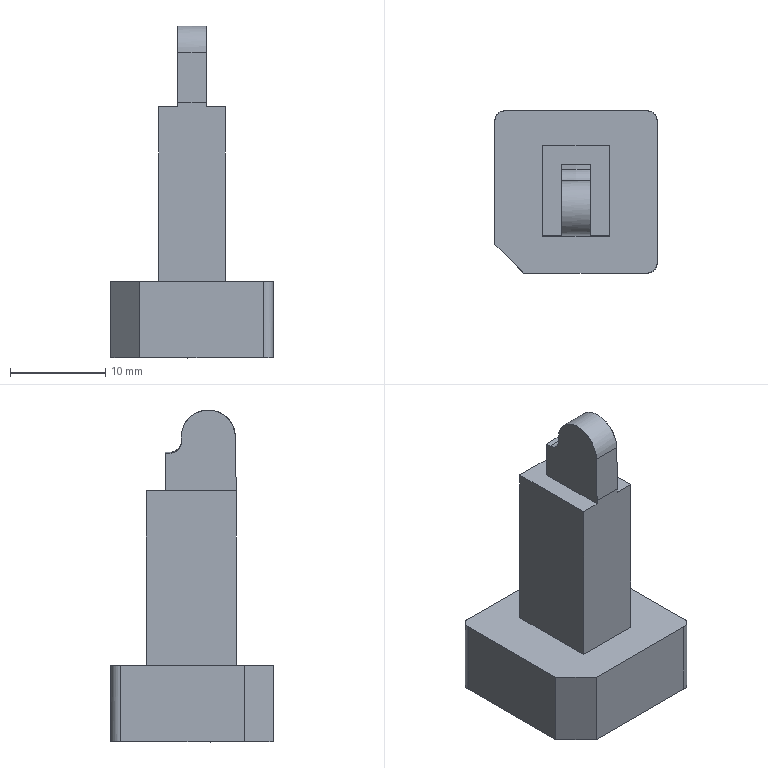NC program | PowerMill | posted with a generic post | part box 17 x 17 x 34.811 mm
Lines 14457 to 15230 of 35253:
N14554 M6
N14555 S18000 M03
N14556 G00 G90 X0.0 Y0.0
N14557 G43 Z10.798 H14
N14558
N14559 G05 P10000 R8
N14560 X2.9016 Y-3.9127
N14561 Z0.8984
N14562 G01 Z-0.3016 F1200.0
N14563 X2.8751 Y-3.8463 F2000.0
N14564 X2.8414 Y-3.7833
N14565 X2.8009 Y-3.7245
N14566 X2.7541 Y-3.6705
N14567 X2.7015 Y-3.6221
N14568 X2.6439 Y-3.5798
N14569 X2.582 Y-3.5442
N14570 X2.5165 Y-3.5158
N14571 X2.4482 Y-3.4948
N14572 X2.378 Y-3.4816
N14573 X2.3067 Y-3.4763
N14574 X2.2353 Y-3.479
N14575 X2.1646 Y-3.4896
N14576 X2.0956 Y-3.508
N14577 X2.0913 Y-3.5094
N14578 X2.0196 Y-3.5335
N14579 X1.935 Y-3.558
N14580 X1.861 Y-3.5731
N14581 X1.7759 Y-3.5869
N14582 X1.6905 Y-3.5984
N14583 X1.6048 Y-3.6064
N14584 X1.5186 Y-3.6099
N14585 X1.4322 Y-3.6102
N14586 X1.3457 Y-3.6093
N14587 X1.2593 Y-3.6087
N14588 X1.173 Y-3.6086
N14589 X-0.307 Y-3.6083
N14590 X-1.5504 Y-3.6069
N14591 X-1.6606 Y-3.6026
N14592 X-1.7723 Y-3.5904
N14593 X-1.8848 Y-3.5701
N14594 X-1.9976 Y-3.5416
N14595 X-2.1099 Y-3.5051
N14596 X-2.221 Y-3.4607
N14597 X-2.33 Y-3.4085
N14598 X-2.4359 Y-3.3489
N14599 X-2.5297 Y-3.2881
N14600 X-2.6248 Y-3.2174
N14601 X-2.7156 Y-3.1401
N14602 X-2.8014 Y-3.0565
N14603 X-2.8816 Y-2.9672
N14604 X-2.9556 Y-2.873
N14605 X-3.0196 Y-2.7794
N14606 X-3.0808 Y-2.6764
N14607 X-3.1339 Y-2.5718
N14608 X-3.1789 Y-2.4664
N14609 X-3.2136 Y-2.3667
N14610 X-3.2381 Y-2.2836
N14611 X-3.2593 Y-2.1999
N14612 X-3.2766 Y-2.1154
N14613 X-3.2893 Y-2.03
N14614 X-3.2981 Y-1.9322
N14615 X-3.3018 Y-1.8219
N14616 X-3.3019 Y-1.7278
N14617 X-3.3008 Y-1.6407
N14618 X-3.2997 Y-1.5539
N14619 X-3.2965 Y-1.4653
N14620 X-3.2853 Y-1.353
N14621 X-3.2661 Y-1.2393
N14622 X-3.2386 Y-1.1245
N14623 X-3.2029 Y-1.0088
N14624 X-3.1594 Y-0.8944
N14625 X-3.1149 Y-0.796
N14626 X-3.0684 Y-0.7098
N14627 X-3.0192 Y-0.6338
N14628 X-2.9764 Y-0.5739
N14629 X-2.9331 Y-0.5143
N14630 X-2.8889 Y-0.4555
N14631 X-2.8426 Y-0.3983
N14632 X-2.7926 Y-0.3443
N14633 X-2.7388 Y-0.2938
N14634 X-2.6837 Y-0.2448
N14635 X-2.6276 Y-0.1972
N14636 X-2.5426 Y-0.1328
N14637 X-2.4457 Y-0.0685
N14638 X-2.3401 Y-0.0078
N14639 X-2.2358 Y0.0436
N14640 X-2.1366 Y0.0848
N14641 X-2.0402 Y0.1172
N14642 X-1.9499 Y0.1419
N14643 X-1.8588 Y0.1627
N14644 X-1.7668 Y0.1788
N14645 X-1.6637 Y0.1909
N14646 X-1.5428 Y0.1983
N14647 X-1.4385 Y0.2005
N14648 X-1.3444 Y0.2008
N14649 X-1.2505 Y0.2005
N14650 X-1.1548 Y0.2002
N14651 X0.8185 Y0.1975
N14652 X1.5507 Y0.1972
N14653 X1.6544 Y0.1933
N14654 X1.7622 Y0.1813
N14655 X1.8739 Y0.1611
N14656 X1.9893 Y0.1322
N14657 X2.1076 Y0.0946
N14658 X2.208 Y0.0563
N14659 X2.3058 Y0.012
N14660 X2.4032 Y-0.0409
N14661 X2.501 Y-0.1028
N14662 X2.5993 Y-0.1742
N14663 X2.6925 Y-0.2508
N14664 X2.7784 Y-0.3305
N14665 X2.8591 Y-0.4163
N14666 X2.9341 Y-0.5078
N14667 X3.0032 Y-0.6044
N14668 X3.0657 Y-0.7058
N14669 X3.1214 Y-0.8113
N14670 X3.1699 Y-0.92
N14671 X3.2109 Y-1.0316
N14672 X3.2442 Y-1.1453
N14673 X3.2697 Y-1.2606
N14674 X3.2874 Y-1.3769
N14675 X3.2972 Y-1.4936
N14676 X3.3 Y-1.5974
N14677 X3.3022 Y-1.7022
N14678 X3.3029 Y-1.8212
N14679 X3.2989 Y-1.9403
N14680 X3.2898 Y-2.0396
N14681 X3.2765 Y-2.1274
N14682 X3.2581 Y-2.2141
N14683 X3.2353 Y-2.2998
N14684 X3.2084 Y-2.3846
N14685 X3.1781 Y-2.4684
N14686 X3.1357 Y-2.5677
N14687 X3.0838 Y-2.6695
N14688 X3.0214 Y-2.7749
N14689 X2.9546 Y-2.8732
N14690 X2.8812 Y-2.9671
N14691 X2.8016 Y-3.0559
N14692 X2.7163 Y-3.1392
N14693 X2.6255 Y-3.2166
N14694 X2.5297 Y-3.2879
N14695 X2.4294 Y-3.3525
N14696 X2.325 Y-3.4103
N14697 X2.2171 Y-3.4609
N14698 X2.106 Y-3.5043
N14699 X2.0913 Y-3.5094
N14700 X2.0478 Y-3.5263
N14701 X1.9916 Y-3.545 Z-0.3017
N14702 X1.9468 Y-3.5583
N14703 X1.9017 Y-3.5701 Z-0.3018
N14704 X1.8559 Y-3.579
N14705 X1.7465 Y-3.5975 Z-0.302
N14706 X1.6366 Y-3.6124 Z-0.3021
N14707 X1.5261 Y-3.6217 Z-0.3022
N14708 X1.4151 Y-3.6257 Z-0.3023
N14709 X1.3041 Y-3.6275 Z-0.3024
N14710 X1.1931 Y-3.629 Z-0.3025
N14711 X0.7459 Y-3.639 Z-0.303
N14712 X0.1167 Y-3.657 Z-0.3037
N14713 X-0.3503 Y-3.6667 Z-0.3041
N14714 X-1.1718 Y-3.6853 Z-0.305
N14715 X-1.5566 Y-3.6938 Z-0.3054
N14716 X-1.6463 Y-3.6921 Z-0.3055
N14717 X-1.7357 Y-3.6845 Z-0.3056
N14718 X-1.8378 Y-3.6699
N14719 X-1.9534 Y-3.6464 Z-0.3058
N14720 X-2.0677 Y-3.6159 Z-0.3059
N14721 X-2.1667 Y-3.5829 Z-0.3061
N14722 X-2.2515 Y-3.5485 Z-0.3063
N14723 X-2.3617 Y-3.4957 Z-0.3065
N14724 X-2.4608 Y-3.4404 Z-0.3068
N14725 X-2.5503 Y-3.3822 Z-0.3069
N14726 X-2.6341 Y-3.3193 Z-0.307
N14727 X-2.7184 Y-3.2495 Z-0.3072
N14728 X-2.8017 Y-3.1719 Z-0.3076
N14729 X-2.8761 Y-3.0927 Z-0.308
N14730 X-2.9429 Y-3.0115 Z-0.3083
N14731 X-3.0047 Y-2.9264 Z-0.3084
N14732 X-3.06 Y-2.8426 Z-0.3087
N14733 X-3.1015 Y-2.7717 Z-0.3092
N14734 X-3.1221 Y-2.7308 Z-0.3093
N14735 X-3.1411 Y-2.6928 Z-0.3098
N14736 X-3.1631 Y-2.6502 Z-0.3111
N14737 X-3.1977 Y-2.5825 Z-0.3135
N14738 X-3.2198 Y-2.5361 Z-0.315
N14739 X-3.236 Y-2.497 Z-0.3159
N14740 X-3.2487 Y-2.4566 Z-0.3163
N14741 X-3.2728 Y-2.3617 Z-0.3169
N14742 X-3.2881 Y-2.2719 Z-0.3173
N14743 X-3.2952 Y-2.1889 Z-0.3176
N14744 X-3.2977 Y-2.1054 Z-0.3179
N14745 X-3.3013 Y-1.8637 Z-0.3183
N14746 X-3.3017 Y-1.622 Z-0.319
N14747 Y-1.3817 Z-0.3195
N14748 X-3.298 Y-1.265 Z-0.3197
N14749 X-3.2863 Y-1.143 Z-0.3202
N14750 X-3.2669 Y-1.0212 Z-0.3205
N14751 X-3.2412 Y-0.9066 Z-0.3207
N14752 X-3.2258 Y-0.8515 Z-0.3206
N14753 X-3.2048 Y-0.7959 Z-0.3197
N14754 X-3.1714 Y-0.7258 Z-0.3177
N14755 X-3.1321 Y-0.6469 Z-0.3161
N14756 X-3.1075 Y-0.5963 Z-0.3159
N14757 X-3.0769 Y-0.5454 Z-0.3152
N14758 X-3.048 Y-0.4971 Z-0.315
N14759 X-2.9865 Y-0.3994 Z-0.3151
N14760 X-2.9167 Y-0.3033 Z-0.3152
N14761 X-2.8391 Y-0.21 Z-0.3154
N14762 X-2.7545 Y-0.1208 Z-0.3157
N14763 X-2.6724 Y-0.0441 Z-0.316
N14764 X-2.5801 Y0.0336 Z-0.3164
N14765 X-2.4999 Y0.0935 Z-0.3168
N14766 X-2.4164 Y0.1485 Z-0.3172
N14767 X-2.3114 Y0.2099 Z-0.3177
N14768 X-2.2085 Y0.2615 Z-0.3181
N14769 X-2.1078 Y0.3038 Z-0.3184
N14770 X-2.0091 Y0.3371 Z-0.3186
N14771 X-1.9189 Y0.3617 Z-0.3188
N14772 X-1.828 Y0.3829 Z-0.319
N14773 X-1.7362 Y0.3998 Z-0.3193
N14774 X-1.6384 Y0.4123 Z-0.3196
N14775 X-1.5372 Y0.4198 Z-0.3199
N14776 X-1.4435 Y0.4233 Z-0.3202
N14777 X-1.3497 Y0.425 Z-0.3204
N14778 X-1.256 Y0.4259 Z-0.3206
N14779 X-1.1625 Y0.427 Z-0.3209
N14780 X-0.7326 Y0.4357 Z-0.3219
N14781 X-0.1421 Y0.4514 Z-0.3235
N14782 X0.3613 Y0.462 Z-0.3248
N14783 X1.3883 Y0.4864 Z-0.3278
N14784 X1.4783 Y0.4881 Z-0.3281
N14785 X1.5685 Y0.488 Z-0.3284
N14786 X1.6585 Y0.485 Z-0.3287
N14787 X1.7483 Y0.4776 Z-0.329
N14788 X1.8373 Y0.4647 Z-0.3293
N14789 X1.9256 Y0.4469 Z-0.3297
N14790 X2.013 Y0.4256 Z-0.33
N14791 X2.1207 Y0.3936 Z-0.3305
N14792 X2.227 Y0.3538 Z-0.3309
N14793 X2.332 Y0.306 Z-0.3313
N14794 X2.4352 Y0.2502 Z-0.3317
N14795 X2.5354 Y0.1873 Z-0.3321
N14796 X2.6313 Y0.1175 Z-0.3324
N14797 X2.7231 Y0.041 Z-0.3329
N14798 X2.8103 Y-0.042 Z-0.3334
N14799 X2.8922 Y-0.1312 Z-0.334
N14800 X2.9686 Y-0.2259 Z-0.3348
N14801 X3.0403 Y-0.3249 Z-0.3365
N14802 X3.0898 Y-0.4002 Z-0.3384
N14803 X3.1269 Y-0.4675 Z-0.3394
N14804 X3.1692 Y-0.5608 Z-0.3399
N14805 X3.2092 Y-0.6673 Z-0.3401
N14806 X3.2432 Y-0.7797 Z-0.3404
N14807 X3.2696 Y-0.8943 Z-0.3407
N14808 X3.2882 Y-1.0108 Z-0.341
N14809 X3.2989 Y-1.1286 Z-0.3413
N14810 X3.3017 Y-1.2473 Z-0.3416
N14811 Y-2.1997 Z-0.3439
N14812 X3.2978 Y-2.3244 Z-0.3443
N14813 X3.2859 Y-2.4476 Z-0.3447
N14814 X3.2663 Y-2.5688 Z-0.3451
N14815 X3.2391 Y-2.6875 Z-0.3454
N14816 X3.2045 Y-2.803 Z-0.3457
N14817 X3.1628 Y-2.9151 Z-0.346
N14818 X3.114 Y-3.0232 Z-0.3462
N14819 X3.0586 Y-3.1271 Z-0.3463
N14820 X2.9965 Y-3.2267
N14821 X2.926 Y-3.3248 Z-0.3464
N14822 X2.8479 Y-3.4199 Z-0.3466
N14823 X2.7631 Y-3.5105 Z-0.347
N14824 X2.6734 Y-3.5949 Z-0.3474
N14825 X2.5798 Y-3.6721 Z-0.3479
N14826 X2.4837 Y-3.7414 Z-0.3484
N14827 X2.3859 Y-3.8025 Z-0.3489
N14828 X2.2875 Y-3.855 Z-0.3493
N14829 X2.2596 Y-3.8682 Z-0.3494
N14830 X2.1901 Y-3.9012 Z-0.3496
N14831 X2.1164 Y-3.9305 Z-0.3497
N14832 X2.0149 Y-3.9647 Z-0.35
N14833 X1.9407 Y-3.9858 Z-0.3501
N14834 X1.8657 Y-4.0034 Z-0.3503
N14835 X1.7538 Y-4.0228 Z-0.3506
N14836 X1.6322 Y-4.0363 Z-0.3508
N14837 X1.494 Y-4.0442 Z-0.3511
N14838 X1.3253 Y-4.0467 Z-0.3515
N14839 X1.0775 Y-4.046 Z-0.3521
N14840 X0.6713 Y-4.0498 Z-0.353
N14841 X0.088 Y-4.0593 Z-0.3543
N14842 X-0.3656 Y-4.0635 Z-0.3553
N14843 X-1.3875 Y-4.0755 Z-0.3575
N14844 X-1.4777 Y-4.076 Z-0.3577
N14845 X-1.5679 Y-4.0747 Z-0.3579
N14846 X-1.658 Y-4.0705 Z-0.3581
N14847 X-1.7478 Y-4.0623 Z-0.3582
N14848 X-1.843 Y-4.048 Z-0.3584
N14849 X-1.9311 Y-4.0292 Z-0.3586
N14850 X-2.0183 Y-4.006 Z-0.3588
N14851 X-2.1044 Y-3.9794 Z-0.359
N14852 X-2.2124 Y-3.9389 Z-0.3592
N14853 X-2.318 Y-3.8908 Z-0.3594
N14854 X-2.4209 Y-3.8352 Z-0.3597
N14855 X-2.5183 Y-3.7739 Z-0.3599
N14856 X-2.6164 Y-3.7034 Z-0.3604
N14857 X-2.7117 Y-3.6256 Z-0.3609
N14858 X-2.7982 Y-3.5452 Z-0.3614
N14859 X-2.8742 Y-3.4647 Z-0.3619
N14860 X-2.9394 Y-3.3853 Z-0.3623
N14861 X-2.9993 Y-3.3016 Z-0.3627
N14862 X-3.0635 Y-3.1993 Z-0.363
N14863 X-3.1204 Y-3.0938 Z-0.3634
N14864 X-3.1696 Y-2.9858 Z-0.3637
N14865 X-3.211 Y-2.8759 Z-0.3639
N14866 X-3.2445 Y-2.7646 Z-0.3642
N14867 X-3.2701 Y-2.6523 Z-0.3644
N14868 X-3.2877 Y-2.5396 Z-0.3647
N14869 X-3.2974 Y-2.4268 Z-0.365
N14870 X-3.3 Y-2.3136 Z-0.3652
N14871 X-3.3036 Y-1.727 Z-0.3667
N14872 X-3.3015 Y-1.0608 Z-0.3683
N14873 X-3.2968 Y-0.948 Z-0.3685
N14874 X-3.2841 Y-0.8338 Z-0.3688
N14875 X-3.2634 Y-0.7183 Z-0.3691
N14876 X-3.2345 Y-0.6018 Z-0.3694
N14877 X-3.1972 Y-0.4849 Z-0.3697
N14878 X-3.1536 Y-0.3726 Z-0.3699
N14879 X-3.1033 Y-0.264 Z-0.3703
N14880 X-3.0464 Y-0.16 Z-0.3707
N14881 X-2.9832 Y-0.061 Z-0.3709
N14882 X-2.9141 Y0.033
N14883 X-2.8379 Y0.1234 Z-0.371
N14884 X-2.7559 Y0.2085
N14885 X-2.668 Y0.2882 Z-0.3711
N14886 X-2.574 Y0.3627 Z-0.3712
N14887 X-2.4738 Y0.4319 Z-0.3713
N14888 X-2.3735 Y0.4925 Z-0.3715
N14889 X-2.2668 Y0.5485 Z-0.3718
N14890 X-2.1585 Y0.5964 Z-0.3721
N14891 X-2.0487 Y0.6365 Z-0.3724
N14892 X-1.9369 Y0.6688 Z-0.3727
N14893 X-1.8301 Y0.6922 Z-0.373
N14894 X-1.7157 Y0.7093 Z-0.3733
N14895 X-1.5869 Y0.721 Z-0.3735
N14896 X-1.435 Y0.7275 Z-0.3738
N14897 X-1.2322 Y0.7298 Z-0.3743
N14898 X-0.8657 Y0.7323 Z-0.3752
N14899 X0.3671 Y0.7445 Z-0.3781
N14900 X1.5479 Y0.7569 Z-0.3809
N14901 X1.6453 Y0.7541 Z-0.3812
N14902 X1.7473 Y0.7441 Z-0.3815
N14903 X1.86 Y0.7259 Z-0.3817
N14904 X1.9799 Y0.6987 Z-0.382
N14905 X2.0924 Y0.6658 Z-0.3823
N14906 X2.1914 Y0.6303 Z-0.3825
N14907 X2.2744 Y0.5948 Z-0.3827
N14908 X2.3553 Y0.5544 Z-0.383
N14909 X2.4444 Y0.504 Z-0.3834
N14910 X2.546 Y0.4389 Z-0.384
N14911 X2.6404 Y0.3705 Z-0.3847
N14912 X2.7173 Y0.3076 Z-0.3852
N14913 X2.7834 Y0.2462 Z-0.3856
N14914 X2.8452 Y0.1803 Z-0.3859
N14915 X2.9239 Y0.0858 Z-0.3862
N14916 X2.9958 Y-0.0128 Z-0.3865
N14917 X3.0605 Y-0.1149 Z-0.3868
N14918 X3.1176 Y-0.2198 Z-0.3871
N14919 X3.167 Y-0.3269 Z-0.3874
N14920 X3.2086 Y-0.4357 Z-0.3876
N14921 X3.2422 Y-0.5456 Z-0.3879
N14922 X3.2677 Y-0.6562 Z-0.3882
N14923 X3.2853 Y-0.7671 Z-0.3884
N14924 X3.295 Y-0.8781 Z-0.3887
N14925 X3.2987 Y-0.9897 Z-0.389
N14926 X3.3018 Y-1.1756 Z-0.3895
N14927 X3.3033 Y-1.3615 Z-0.3899
N14928 X3.3039 Y-1.5475 Z-0.3904
N14929 X3.3037 Y-1.7631 Z-0.3909
N14930 X3.303 Y-1.9491 Z-0.3913
N14931 X3.3018 Y-2.135 Z-0.3917
N14932 X3.3 Y-2.321 Z-0.3922
N14933 X3.2974 Y-2.507 Z-0.3926
N14934 X3.2935 Y-2.607 Z-0.3929
N14935 X3.282 Y-2.7094 Z-0.3931
N14936 X3.2622 Y-2.8155 Z-0.3934
N14937 X3.2337 Y-2.9257 Z-0.3937
N14938 X3.196 Y-3.0405 Z-0.394
N14939 X3.1486 Y-3.1604 Z-0.3943
N14940 X3.1005 Y-3.2638 Z-0.3945
N14941 X3.0448 Y-3.3647 Z-0.3948
N14942 X2.9814 Y-3.4633 Z-0.3951
N14943 X2.9103 Y-3.5592 Z-0.3954
N14944 X2.8317 Y-3.6519 Z-0.3957
N14945 X2.7457 Y-3.7411 Z-0.396
N14946 X2.687 Y-3.7959 Z-0.3962
N14947 X2.6257 Y-3.8478 Z-0.3963
N14948 X2.5588 Y-3.8991 Z-0.3965
N14949 X2.4701 Y-3.9606 Z-0.3968
N14950 X2.4019 Y-4.0027 Z-0.397
N14951 X2.3404 Y-4.0357 Z-0.3972
N14952 X2.2407 Y-4.0857 Z-0.3974
N14953 X2.1331 Y-4.1311 Z-0.3977
N14954 X2.0196 Y-4.1705 Z-0.3979
N14955 X1.9044 Y-4.2021 Z-0.3982
N14956 X1.7905 Y-4.2254 Z-0.3984
N14957 X1.68 Y-4.2403 Z-0.3987
N14958 X1.5741 Y-4.2472 Z-0.3989
N14959 X1.4685 Y-4.2487 Z-0.3991
N14960 X0.3105 Y-4.2597 Z-0.4016
N14961 X-1.0396 Y-4.2704 Z-0.4045
N14962 X-1.3875 Y-4.2737 Z-0.4052
N14963 X-1.4804 Y-4.2742 Z-0.4054
N14964 X-1.5734 Y-4.2729 Z-0.4057
N14965 X-1.6726 Y-4.2679 Z-0.406
N14966 X-1.7789 Y-4.2567 Z-0.4063
N14967 X-1.8702 Y-4.2411 Z-0.4065
N14968 X-1.9604 Y-4.2202 Z-0.4067
N14969 X-2.0495 Y-4.1947 Z-0.4068
N14970 X-2.1374 Y-4.1651 Z-0.4069
N14971 X-2.2475 Y-4.1209 Z-0.4072
N14972 X-2.3547 Y-4.0694 Z-0.4076
N14973 X-2.459 Y-4.0104 Z-0.408
N14974 X-2.5552 Y-3.9476 Z-0.4085
N14975 X-2.6469 Y-3.879 Z-0.409
N14976 X-2.7329 Y-3.8048 Z-0.4094
N14977 X-2.8178 Y-3.7211 Z-0.4096
N14978 X-2.8962 Y-3.6327 Z-0.4099
N14979 X-2.9676 Y-3.5403 Z-0.4102
N14980 X-3.032 Y-3.4442 Z-0.4104
N14981 X-3.0822 Y-3.3575 Z-0.4107
N14982 X-3.1382 Y-3.2481 Z-0.411
N14983 X-3.1799 Y-3.1535 Z-0.4112
N14984 X-3.2116 Y-3.0651 Z-0.4114
N14985 X-3.2378 Y-2.9778 Z-0.4116
N14986 X-3.2598 Y-2.8885 Z-0.4118
N14987 X-3.2775 Y-2.7948 Z-0.4121
N14988 X-3.2907 Y-2.6926 Z-0.4123
N14989 X-3.299 Y-2.5745 Z-0.4126
N14990 X-3.3021 Y-2.4384 Z-0.413
N14991 X-3.302 Y-2.3197 Z-0.4132
N14992 X-3.3016 Y-2.2106 Z-0.4134
N14993 Y-2.0981 Z-0.4136
N14994 X-3.3017 Y-0.8977 Z-0.4165
N14995 X-3.2977 Y-0.7794 Z-0.4167
N14996 X-3.2858 Y-0.6615 Z-0.417
N14997 X-3.2659 Y-0.5441 Z-0.4173
N14998 X-3.2382 Y-0.4277 Z-0.4176
N14999 X-3.2026 Y-0.3129 Z-0.4179
N15000 X-3.1593 Y-0.2001 Z-0.4182
N15001 X-3.1084 Y-0.0901 Z-0.4185
N15002 X-3.0503 Y0.0168 Z-0.4187
N15003 X-2.9852 Y0.1197 Z-0.419
N15004 X-2.9143 Y0.2169 Z-0.4192
N15005 X-2.8372 Y0.3092 Z-0.4195
N15006 X-2.7544 Y0.3958 Z-0.4199
N15007 X-2.6663 Y0.4765 Z-0.4202
N15008 X-2.5735 Y0.5507 Z-0.4204
N15009 X-2.4765 Y0.6182 Z-0.4206
N15010 X-2.3751 Y0.6791 Z-0.4207
N15011 X-2.2678 Y0.7343 Z-0.4208
N15012 X-2.1565 Y0.7826 Z-0.421
N15013 X-2.0425 Y0.8234 Z-0.4212
N15014 X-1.9274 Y0.8562 Z-0.4214
N15015 X-1.8123 Y0.8809 Z-0.4216
N15016 X-1.6982 Y0.8975 Z-0.4219
N15017 X-1.586 Y0.9059 Z-0.4221
N15018 X-1.4744 Y0.9083 Z-0.4224
N15019 X-0.9294 Y0.9139 Z-0.4237
N15020 X-0.317 Y0.918 Z-0.4251
N15021 X0.7133 Y0.9251 Z-0.4276
N15022 X1.4557 Y0.9316 Z-0.4294
N15023 X1.5869 Y0.9296 Z-0.4297
N15024 X1.7121 Y0.9203 Z-0.43
N15025 X1.832 Y0.904 Z-0.4303
N15026 X1.9472 Y0.8805 Z-0.4306
N15027 X2.0581 Y0.85 Z-0.431
N15028 X2.1655 Y0.8125 Z-0.4314
N15029 X2.2707 Y0.7679 Z-0.4318
N15030 X2.3778 Y0.714 Z-0.4322
N15031 X2.4806 Y0.6534 Z-0.4325
N15032 X2.5787 Y0.5863 Z-0.4328
N15033 X2.6717 Y0.5131 Z-0.433
N15034 X2.7592 Y0.434 Z-0.4332
N15035 X2.8412 Y0.3493 Z-0.4335
N15036 X2.9172 Y0.2595 Z-0.4338
N15037 X2.9888 Y0.1625 Z-0.4341
N15038 X3.0536 Y0.0613 Z-0.4344
N15039 X3.1113 Y-0.0434 Z-0.4347
N15040 X3.1616 Y-0.151 Z-0.4349
N15041 X3.2041 Y-0.261 Z-0.4352
N15042 X3.2389 Y-0.3726 Z-0.4355
N15043 X3.2658 Y-0.4855 Z-0.4357
N15044 X3.2847 Y-0.599 Z-0.436
N15045 X3.2957 Y-0.7126 Z-0.4363
N15046 X3.3005 Y-0.8269 Z-0.4365
N15047 X3.3041 Y-1.048 Z-0.4371
N15048 X3.3028 Y-1.3477 Z-0.4377
N15049 X3.3017 Y-1.664 Z-0.4385
N15050 Y-2.2037 Z-0.4397
N15051 X3.2993 Y-2.6465 Z-0.4408
N15052 X3.2985 Y-2.7111 Z-0.4409
N15053 X3.2938 Y-2.7754 Z-0.4411
N15054 X3.2855 Y-2.8405 Z-0.4412
N15055 X3.2709 Y-2.9255 Z-0.4414
N15056 X3.2482 Y-3.0298 Z-0.4417
N15057 X3.2287 Y-3.1042 Z-0.4418
N15058 X3.2095 Y-3.1658 Z-0.442
N15059 X3.1874 Y-3.2265 Z-0.4421
N15060 X3.1382 Y-3.3444 Z-0.4424
N15061 X3.0841 Y-3.4546 Z-0.4427
N15062 X3.0245 Y-3.5587 Z-0.443
N15063 X2.9608 Y-3.6544 Z-0.4433
N15064 X2.8894 Y-3.7475 Z-0.4436
N15065 X2.8106 Y-3.837 Z-0.4438
N15066 X2.7253 Y-3.9221 Z-0.4441
N15067 X2.6347 Y-4.001 Z-0.4444
N15068 X2.5402 Y-4.0731 Z-0.4447
N15069 X2.4427 Y-4.1375 Z-0.4449
N15070 X2.4152 Y-4.1541 Z-0.445
N15071 X2.3065 Y-4.214 Z-0.4453
N15072 X2.2006 Y-4.264 Z-0.4455
N15073 X2.0968 Y-4.3047 Z-0.4458
N15074 X2.0049 Y-4.3342 Z-0.446
N15075 X1.9118 Y-4.359 Z-0.4462
N15076 X1.8177 Y-4.3791 Z-0.4464
N15077 X1.7226 Y-4.3938 Z-0.4466
N15078 X1.6149 Y-4.4041 Z-0.4469
N15079 X1.4917 Y-4.4092 Z-0.4471
N15080 X1.3845 Y-4.41 Z-0.4474
N15081 X1.2854 Y-4.4095 Z-0.4476
N15082 X1.1889 Y-4.4094 Z-0.4478
N15083 X0.9803 Y-4.4105 Z-0.4483
N15084 X0.7717 Y-4.4124 Z-0.4488
N15085 X0.5631 Y-4.4144 Z-0.4492
N15086 X0.3247 Y-4.4168 Z-0.4498
N15087 X0.1161 Y-4.4187 Z-0.4502
N15088 X-0.0925 Y-4.4203 Z-0.4507
N15089 X-0.3011 Y-4.4213 Z-0.4511
N15090 X-1.4563 Y-4.4278 Z-0.4537
N15091 X-1.5595 Y-4.4282 Z-0.4539
N15092 X-1.6625 Y-4.4244 Z-0.4542
N15093 X-1.7697 Y-4.4125 Z-0.4544
N15094 X-1.882 Y-4.3924 Z-0.4547
N15095 X-2.0003 Y-4.3633 Z-0.455
N15096 X-2.1112 Y-4.3291 Z-0.4553
N15097 X-2.2197 Y-4.2875 Z-0.4556
N15098 X-2.3258 Y-4.2383 Z-0.4559
N15099 X-2.429 Y-4.1818 Z-0.4562
N15100 X-2.5288 Y-4.1179 Z-0.4565
N15101 X-2.6249 Y-4.0471 Z-0.4567
N15102 X-2.7167 Y-3.9694 Z-0.457
N15103 X-2.8038 Y-3.8853 Z-0.4573
N15104 X-2.8821 Y-3.7991 Z-0.4575
N15105 X-2.9549 Y-3.7072 Z-0.4578
N15106 X-3.0217 Y-3.6099 Z-0.458
N15107 X-3.0821 Y-3.508 Z-0.4583
N15108 X-3.1354 Y-3.4022 Z-0.4586
N15109 X-3.1747 Y-3.3108 Z-0.4588
N15110 X-3.2085 Y-3.2196 Z-0.459
N15111 X-3.2375 Y-3.1252 Z-0.4592
N15112 X-3.2615 Y-3.0257 Z-0.4595
N15113 X-3.2804 Y-2.9179 Z-0.4597
N15114 X-3.2937 Y-2.7983 Z-0.46
N15115 X-3.3011 Y-2.6676 Z-0.4603
N15116 X-3.3036 Y-2.5423 Z-0.4606
N15117 X-3.3038 Y-2.4223 Z-0.4609
N15118 X-3.3033 Y-2.3054 Z-0.4611
N15119 X-3.303 Y-2.1853 Z-0.4614
N15120 X-3.3016 Y-0.7345 Z-0.4647
N15121 X-3.2976 Y-0.6215 Z-0.4649
N15122 X-3.2857 Y-0.5077 Z-0.4652
N15123 X-3.2657 Y-0.3932 Z-0.4654
N15124 X-3.2376 Y-0.2784 Z-0.4657
N15125 X-3.2014 Y-0.1637 Z-0.466
N15126 X-3.1571 Y-0.0497 Z-0.4663
N15127 X-3.1048 Y0.0629 Z-0.4665
N15128 X-3.0479 Y0.1672 Z-0.4668
N15129 X-2.9839 Y0.2677 Z-0.4671
N15130 X-2.9132 Y0.3642 Z-0.4673
N15131 X-2.8359 Y0.456 Z-0.4676
N15132 X-2.7524 Y0.5427 Z-0.4679
N15133 X-2.6632 Y0.6239 Z-0.4682
N15134 X-2.5689 Y0.699 Z-0.4684
N15135 X-2.4708 Y0.767 Z-0.4687
N15136 X-2.3694 Y0.8277 Z-0.469
N15137 X-2.2652 Y0.881 Z-0.4692
N15138 X-2.1761 Y0.9197 Z-0.4695
N15139 X-2.088 Y0.953 Z-0.4697
N15140 X-1.9984 Y0.9821 Z-0.4699
N15141 X-1.9051 Y1.007 Z-0.4701
N15142 X-1.8052 Y1.0274 Z-0.4703
N15143 X-1.6942 Y1.0429 Z-0.4706
N15144 X-1.5686 Y1.0528 Z-0.4709
N15145 X-1.4502 Y1.057 Z-0.4711
N15146 X-1.3386 Y1.0581 Z-0.4714
N15147 X-1.2307 Y1.0582 Z-0.4716
N15148 X-1.1192 Z-0.4719
N15149 X-0.3132 Y1.0615 Z-0.4737
N15150 X0.4996 Y1.0667 Z-0.4755
N15151 X0.9845 Y1.0712 Z-0.4766
N15152 X1.384 Y1.0733 Z-0.4775
N15153 X1.5593 Y1.072 Z-0.4779
N15154 X1.6704 Y1.0667 Z-0.4782
N15155 X1.7831 Y1.0534 Z-0.4784
N15156 X1.8974 Y1.0319 Z-0.4787
N15157 X2.0128 Y1.0022 Z-0.479
N15158 X2.1289 Y0.9642 Z-0.4792
N15159 X2.2377 Y0.9209 Z-0.4795
N15160 X2.3435 Y0.8705 Z-0.4798
N15161 X2.4463 Y0.8127 Z-0.48
N15162 X2.5456 Y0.7477 Z-0.4803
N15163 X2.6409 Y0.6758 Z-0.4806
N15164 X2.7317 Y0.5973 Z-0.4809
N15165 X2.8167 Y0.5135 Z-0.4811
N15166 X2.8946 Y0.4257 Z-0.4814
N15167 X2.9652 Y0.3344 Z-0.4816
N15168 X3.0283 Y0.2401 Z-0.4819
N15169 X3.085 Y0.1418 Z-0.4822
N15170 X3.1383 Y0.0343 Z-0.4824
N15171 X3.1895 Y-0.0854 Z-0.4827
N15172 X3.2095 Y-0.1414 Z-0.4829
N15173 X3.2269 Y-0.1982 Z-0.483
N15174 X3.2457 Y-0.267 Z-0.4832
N15175 X3.2687 Y-0.3653 Z-0.4834
N15176 X3.2838 Y-0.4461 Z-0.4836
N15177 X3.2923 Y-0.5075 Z-0.4837
N15178 X3.2965 Y-0.5666 Z-0.4838
N15179 X3.2973 Y-0.626 Z-0.484
N15180 X3.3015 Y-0.9821 Z-0.4848
N15181 X3.3017 Y-1.2945 Z-0.4855
N15182 Y-1.714 Z-0.4864
N15183 X3.3025 Y-2.3333 Z-0.4878
N15184 X3.2998 Y-2.7236 Z-0.4887
N15185 X3.2974 Y-2.8584 Z-0.489
N15186 X3.2934 Y-2.9164 Z-0.4892
N15187 X3.2859 Y-2.9741 Z-0.4893
N15188 X3.2741 Y-3.0443 Z-0.4895
N15189 X3.2539 Y-3.1413 Z-0.4897
N15190 X3.2324 Y-3.227 Z-0.4899
N15191 X3.214 Y-3.29 Z-0.49
N15192 X3.1951 Y-3.3451 Z-0.4902
N15193 X3.1736 Y-3.3993 Z-0.4903
N15194 X3.1218 Y-3.5153 Z-0.4906
N15195 X3.0641 Y-3.6253 Z-0.4909
N15196 X3.0105 Y-3.7142 Z-0.4911
N15197 X2.9591 Y-3.7893 Z-0.4913
N15198 X2.8954 Y-3.8717 Z-0.4915
N15199 X2.8183 Y-3.9602 Z-0.4918
N15200 X2.7327 Y-4.0471 Z-0.4921
N15201 X2.6501 Y-4.1211 Z-0.4923
N15202 X2.5729 Y-4.182 Z-0.4925
N15203 X2.4991 Y-4.2326 Z-0.4927
N15204 X2.4733 Y-4.2483 Z-0.4928
N15205 X2.371 Y-4.311 Z-0.4931
N15206 X2.2656 Y-4.3663 Z-0.4933
N15207 X2.1571 Y-4.4143 Z-0.4936
N15208 X2.0458 Y-4.4548 Z-0.4939
N15209 X1.9447 Y-4.4838 Z-0.4941
N15210 X1.8359 Y-4.507 Z-0.4943
N15211 X1.7169 Y-4.5245 Z-0.4946
N15212 X1.5842 Y-4.5364 Z-0.4949
N15213 X1.4309 Y-4.5427 Z-0.4952
N15214 X1.239 Y-4.5439 Z-0.4957
N15215 X0.9371 Y-4.5431 Z-0.4963
N15216 X0.2883 Y-4.5463 Z-0.4978
N15217 X-0.8152 Y-4.5537 Z-0.5002
N15218 X-1.5522 Y-4.5557 Z-0.5018
N15219 X-1.6608 Y-4.5517 Z-0.5021
N15220 X-1.7713 Y-4.5398 Z-0.5023
N15221 X-1.8838 Y-4.5198 Z-0.5026
N15222 X-1.998 Y-4.4914 Z-0.5028
N15223 X-2.1133 Y-4.4547 Z-0.5031
N15224 X-2.222 Y-4.4125 Z-0.5034
N15225 X-2.3278 Y-4.3635 Z-0.5036
N15226 X-2.4307 Y-4.307 Z-0.5039
N15227 X-2.5303 Y-4.2432 Z-0.5041
N15228 X-2.6262 Y-4.1724 Z-0.5044
N15229 X-2.717 Y-4.0955 Z-0.5047
N15230 X-2.8026 Y-4.0127 Z-0.5049
N15231 X-2.8825 Y-3.9242 Z-0.5052
N15232 X-2.9564 Y-3.8306 Z-0.5055
N15233 X-3.0237 Y-3.7323 Z-0.5057
N15234 X-3.0842 Y-3.6299 Z-0.506
N15235 X-3.139 Y-3.5216 Z-0.5062
N15236 X-3.1857 Y-3.4122 Z-0.5065
N15237 X-3.2242 Y-3.3022 Z-0.5068
N15238 X-3.2545 Y-3.1922 Z-0.507
N15239 X-3.2766 Y-3.0825 Z-0.5073
N15240 X-3.2907 Y-2.9735 Z-0.5075
N15241 X-3.2968 Y-2.8654 Z-0.5077
N15242 X-3.298 Y-2.757 Z-0.508
N15243 X-3.3013 Y-2.1048 Z-0.5094
N15244 X-3.3015 Y-1.7139 Z-0.5103
N15245 X-3.3036 Y-1.1977 Z-0.5114
N15246 X-3.3035 Y-0.7848 Z-0.5123
N15247 X-3.3006 Y-0.5704 Z-0.5128
N15248 X-3.2945 Y-0.4619 Z-0.5131
N15249 X-3.2805 Y-0.3511 Z-0.5133
N15250 X-3.2582 Y-0.238 Z-0.5136
N15251 X-3.2274 Y-0.1225 Z-0.5138
N15252 X-3.188 Y-0.005 Z-0.5141
N15253 X-3.1444 Y0.1033 Z-0.5144
N15254 X-3.0938 Y0.2086 Z-0.5146
N15255 X-3.0356 Y0.3112 Z-0.5149
N15256 X-2.9701 Y0.4108 Z-0.5151
N15257 X-2.8974 Y0.5067 Z-0.5154
N15258 X-2.8196 Y0.5966 Z-0.5157
N15259 X-2.7359 Y0.6813 Z-0.5159
N15260 X-2.6467 Y0.7603 Z-0.5162
N15261 X-2.5521 Y0.8334 Z-0.5165
N15262 X-2.4525 Y0.9004 Z-0.5167
N15263 X-2.3483 Y0.9608 Z-0.517
N15264 X-2.2399 Y1.0144 Z-0.5173
N15265 X-2.1278 Y1.0609 Z-0.5175
N15266 X-2.0273 Y1.0955 Z-0.5178
N15267 X-1.9114 Y1.1279 Z-0.518
N15268 X-1.7985 Y1.1517 Z-0.5183
N15269 X-1.6895 Y1.167 Z-0.5185
N15270 X-1.5848 Y1.1742 Z-0.5188
N15271 X-1.4815 Y1.1752 Z-0.519
N15272 X-0.2563 Y1.1827 Z-0.5217
N15273 X0.5047 Y1.1865 Z-0.5234
N15274 X1.2847 Y1.1916 Z-0.5251
N15275 X1.5511 Y1.192 Z-0.5257
N15276 X1.6576 Y1.188 Z-0.5259
N15277 X1.7667 Y1.1761 Z-0.5262
N15278 X1.8787 Y1.1559 Z-0.5264
N15279 X1.9936 Y1.1273 Z-0.5267
N15280 X2.1115 Y1.0898 Z-0.5269
N15281 X2.2172 Y1.0494 Z-0.5272
N15282 X2.3203 Y1.0023 Z-0.5274
N15283 X2.4216 Y0.9472 Z-0.5277
N15284 X2.5208 Y0.8843 Z-0.528
N15285 X2.6175 Y0.8136 Z-0.5282
N15286 X2.7115 Y0.7351 Z-0.5285
N15287 X2.7953 Y0.6554 Z-0.5287
N15288 X2.8742 Y0.5695 Z-0.529
N15289 X2.9474 Y0.4779 Z-0.5293
N15290 X3.0144 Y0.3815 Z-0.5295
N15291 X3.0743 Y0.2812 Z-0.5298
N15292 X3.121 Y0.1908 Z-0.53
N15293 X3.162 Y0.101 Z-0.5302
N15294 X3.1981 Y0.0096 Z-0.5304
N15295 X3.2293 Y-0.0844 Z-0.5307
N15296 X3.2552 Y-0.1829 Z-0.5309
N15297 X3.2759 Y-0.2884 Z-0.5311
N15298 X3.291 Y-0.4041 Z-0.5314
N15299 X3.3003 Y-0.5335 Z-0.5317
N15300 X3.304 Y-0.6693 Z-0.532
N15301 X3.3044 Y-0.7991 Z-0.5322
N15302 X3.3038 Y-0.8987 Z-0.5325
N15303 X3.3012 Y-1.7746 Z-0.5344
N15304 X3.3016 Y-2.6505 Z-0.5363
N15305 X3.3017 Y-2.8605 Z-0.5368
N15306 X3.2978 Y-2.9721 Z-0.5371
N15307 X3.286 Y-3.0865 Z-0.5373
N15308 X3.266 Y-3.2031 Z-0.5376
N15309 X3.2379 Y-3.3206 Z-0.5378
N15310 X3.2019 Y-3.4372 Z-0.5381
N15311 X3.1585 Y-3.5506 Z-0.5384
N15312 X3.1085 Y-3.6595 Z-0.5386
N15313 X3.0526 Y-3.7626 Z-0.5389
N15314 X2.9912 Y-3.8598 Z-0.5392
N15315 X2.9201 Y-3.9572 Z-0.5394
N15316 X2.8424 Y-4.0502 Z-0.5397
N15317 X2.7592 Y-4.1375 Z-0.54
N15318 X2.6714 Y-4.2182 Z-0.5402
N15319 X2.5801 Y-4.2915 Z-0.5405
N15320 X2.5246 Y-4.3314 Z-0.5406
N15321 X2.4217 Y-4.3976 Z-0.5409
N15322 X2.3154 Y-4.4567 Z-0.5412
N15323 X2.2062 Y-4.5082 Z-0.5414
N15324 X2.0949 Y-4.552 Z-0.5417
N15325 X1.9821 Y-4.588 Z-0.5419
N15326 X1.8685 Y-4.6159 Z-0.5422
N15327 X1.7546 Y-4.6358 Z-0.5424